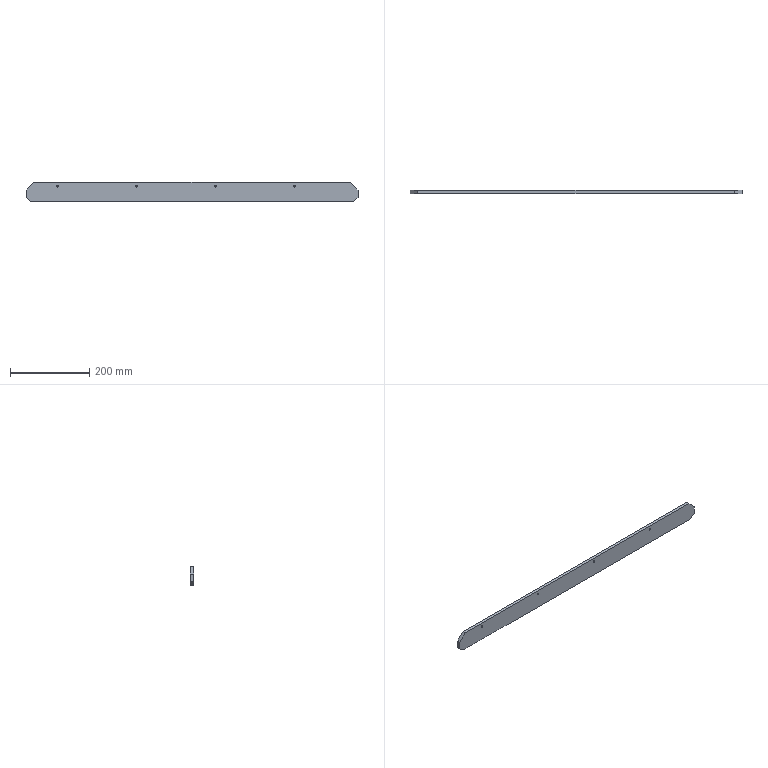Part | STEP file | PN_0038_chain guide rail_default_machined_ | 1 solid | 18 faces | box 840 x 8 x 50 mm | volume 330972 mm3 | plane 10 | cylinder 8 | commonest cylinder face diameters 5 x8
STEP:
#1=CARTESIAN_POINT('',(0.,0.,0.));
#2=DIRECTION('',(0.,0.,1.));
#3=DIRECTION('',(1.,0.,0.));
#4=AXIS2_PLACEMENT_3D('',#1,#2,#3);
#5=CARTESIAN_POINT('',(680.,-8.,-7.5));
#6=VERTEX_POINT('',#5);
#7=CARTESIAN_POINT('',(680.,0.,-7.5));
#8=VERTEX_POINT('',#7);
#9=CARTESIAN_POINT('',(680.,0.,-7.5));
#10=DIRECTION('',(0.,1.,0.));
#11=VECTOR('',#10,1.);
#12=LINE('',#9,#11);
#13=CARTESIAN_POINT('',(680.,0.,-10.));
#14=DIRECTION('',(0.,1.,0.));
#15=DIRECTION('',(0.,0.,1.));
#16=AXIS2_PLACEMENT_3D('',#13,#14,#15);
#17=CYLINDRICAL_SURFACE('',#16,2.5);
#18=CARTESIAN_POINT('',(6.283,0.));
#19=DIRECTION('',(0.,1.));
#20=VECTOR('',#19,1.);
#21=LINE('',#18,#20);
#22=(GEOMETRIC_REPRESENTATION_CONTEXT(2)PARAMETRIC_REPRESENTATION_CONTEXT()REPRESENTATION_CONTEXT('',''));
#23=DEFINITIONAL_REPRESENTATION('',(#21),#22);
#24=PCURVE('',#17,#23);
#25=CARTESIAN_POINT('',(680.,0.,-10.));
#26=DIRECTION('',(0.,1.,0.));
#27=DIRECTION('',(0.,0.,1.));
#28=AXIS2_PLACEMENT_3D('',#25,#26,#27);
#29=CYLINDRICAL_SURFACE('',#28,2.5);
#30=CARTESIAN_POINT('',(0.,0.));
#31=DIRECTION('',(0.,1.));
#32=VECTOR('',#31,1.);
#33=LINE('',#30,#32);
#34=(GEOMETRIC_REPRESENTATION_CONTEXT(2)PARAMETRIC_REPRESENTATION_CONTEXT()REPRESENTATION_CONTEXT('',''));
#35=DEFINITIONAL_REPRESENTATION('',(#33),#34);
#36=PCURVE('',#29,#35);
#37=SURFACE_CURVE('',#12,(#24,#36),.PCURVE_S1.);
#38=EDGE_CURVE('',#6,#8,#37,.T.);
#39=ORIENTED_EDGE('',*,*,#38,.T.);
#40=CARTESIAN_POINT('',(680.,0.,-12.5));
#41=VERTEX_POINT('',#40);
#42=CARTESIAN_POINT('',(680.,0.,-10.));
#43=DIRECTION('',(0.,-1.,0.));
#44=DIRECTION('',(0.,0.,1.));
#45=AXIS2_PLACEMENT_3D('',#42,#43,#44);
#46=CIRCLE('',#45,2.5);
#47=CARTESIAN_POINT('',(6.283,0.));
#48=DIRECTION('',(-1.,0.));
#49=VECTOR('',#48,1.);
#50=LINE('',#47,#49);
#51=(GEOMETRIC_REPRESENTATION_CONTEXT(2)PARAMETRIC_REPRESENTATION_CONTEXT()REPRESENTATION_CONTEXT('',''));
#52=DEFINITIONAL_REPRESENTATION('',(#50),#51);
#53=PCURVE('',#17,#52);
#54=CARTESIAN_POINT('',(0.,0.,0.));
#55=DIRECTION('',(0.,-1.,0.));
#56=DIRECTION('',(0.,0.,-1.));
#57=AXIS2_PLACEMENT_3D('',#54,#55,#56);
#58=PLANE('',#57);
#59=CARTESIAN_POINT('',(10.,680.));
#60=DIRECTION('',(-1.,0.));
#61=AXIS2_PLACEMENT_2D('',#59,#60);
#62=CIRCLE('',#61,2.5);
#63=(GEOMETRIC_REPRESENTATION_CONTEXT(2)PARAMETRIC_REPRESENTATION_CONTEXT()REPRESENTATION_CONTEXT('',''));
#64=DEFINITIONAL_REPRESENTATION('',(#62),#63);
#65=PCURVE('',#58,#64);
#66=SURFACE_CURVE('',#46,(#53,#65),.PCURVE_S1.);
#67=EDGE_CURVE('',#8,#41,#66,.T.);
#68=ORIENTED_EDGE('',*,*,#67,.T.);
#69=CARTESIAN_POINT('',(680.,-8.,-12.5));
#70=VERTEX_POINT('',#69);
#71=CARTESIAN_POINT('',(680.,0.,-12.5));
#72=DIRECTION('',(0.,1.,0.));
#73=VECTOR('',#72,1.);
#74=LINE('',#71,#73);
#75=CARTESIAN_POINT('',(3.142,0.));
#76=DIRECTION('',(0.,1.));
#77=VECTOR('',#76,1.);
#78=LINE('',#75,#77);
#79=(GEOMETRIC_REPRESENTATION_CONTEXT(2)PARAMETRIC_REPRESENTATION_CONTEXT()REPRESENTATION_CONTEXT('',''));
#80=DEFINITIONAL_REPRESENTATION('',(#78),#79);
#81=PCURVE('',#17,#80);
#82=CARTESIAN_POINT('',(3.142,0.));
#83=DIRECTION('',(0.,1.));
#84=VECTOR('',#83,1.);
#85=LINE('',#82,#84);
#86=(GEOMETRIC_REPRESENTATION_CONTEXT(2)PARAMETRIC_REPRESENTATION_CONTEXT()REPRESENTATION_CONTEXT('',''));
#87=DEFINITIONAL_REPRESENTATION('',(#85),#86);
#88=PCURVE('',#29,#87);
#89=SURFACE_CURVE('',#74,(#81,#88),.PCURVE_S1.);
#90=EDGE_CURVE('',#70,#41,#89,.T.);
#91=ORIENTED_EDGE('',*,*,#90,.F.);
#92=CARTESIAN_POINT('',(680.,-8.,-10.));
#93=DIRECTION('',(0.,1.,0.));
#94=DIRECTION('',(0.,0.,1.));
#95=AXIS2_PLACEMENT_3D('',#92,#93,#94);
#96=CIRCLE('',#95,2.5);
#97=CARTESIAN_POINT('',(0.,-8.));
#98=DIRECTION('',(1.,0.));
#99=VECTOR('',#98,1.);
#100=LINE('',#97,#99);
#101=(GEOMETRIC_REPRESENTATION_CONTEXT(2)PARAMETRIC_REPRESENTATION_CONTEXT()REPRESENTATION_CONTEXT('',''));
#102=DEFINITIONAL_REPRESENTATION('',(#100),#101);
#103=PCURVE('',#17,#102);
#104=CARTESIAN_POINT('',(0.,-8.,0.));
#105=DIRECTION('',(0.,-1.,0.));
#106=DIRECTION('',(0.,0.,-1.));
#107=AXIS2_PLACEMENT_3D('',#104,#105,#106);
#108=PLANE('',#107);
#109=CARTESIAN_POINT('',(7.5,680.));
#110=CARTESIAN_POINT('',(7.5,684.33));
#111=CARTESIAN_POINT('',(11.25,682.165));
#112=CARTESIAN_POINT('',(15.,680.));
#113=CARTESIAN_POINT('',(11.25,677.835));
#114=CARTESIAN_POINT('',(7.5,675.67));
#115=CARTESIAN_POINT('',(7.5,680.));
#116=(BOUNDED_CURVE()B_SPLINE_CURVE(2,(#109,#110,#111,#112,#113,#114,#115),.UNSPECIFIED.,.T.,.F.)B_SPLINE_CURVE_WITH_KNOTS((1,2,2,2,2,1),(-2.094,0.,2.094,4.189,6.283,8.378),.UNSPECIFIED.)CURVE()GEOMETRIC_REPRESENTATION_ITEM()RATIONAL_B_SPLINE_CURVE((1.,0.5,1.,0.5,1.,0.5,1.))REPRESENTATION_ITEM(''));
#117=(GEOMETRIC_REPRESENTATION_CONTEXT(2)PARAMETRIC_REPRESENTATION_CONTEXT()REPRESENTATION_CONTEXT('',''));
#118=DEFINITIONAL_REPRESENTATION('',(#116),#117);
#119=PCURVE('',#108,#118);
#120=SURFACE_CURVE('',#96,(#103,#119),.PCURVE_S1.);
#121=EDGE_CURVE('',#70,#6,#120,.T.);
#122=ORIENTED_EDGE('',*,*,#121,.T.);
#123=EDGE_LOOP('',(#39,#68,#91,#122));
#124=FACE_BOUND('',#123,.F.);
#125=ADVANCED_FACE('',(#124),#17,.F.);
#126=CARTESIAN_POINT('',(480.,-8.,-7.5));
#127=VERTEX_POINT('',#126);
#128=CARTESIAN_POINT('',(480.,0.,-7.5));
#129=VERTEX_POINT('',#128);
#130=CARTESIAN_POINT('',(480.,0.,-7.5));
#131=DIRECTION('',(0.,1.,0.));
#132=VECTOR('',#131,1.);
#133=LINE('',#130,#132);
#134=CARTESIAN_POINT('',(480.,0.,-10.));
#135=DIRECTION('',(0.,1.,0.));
#136=DIRECTION('',(0.,0.,1.));
#137=AXIS2_PLACEMENT_3D('',#134,#135,#136);
#138=CYLINDRICAL_SURFACE('',#137,2.5);
#139=CARTESIAN_POINT('',(6.283,0.));
#140=DIRECTION('',(0.,1.));
#141=VECTOR('',#140,1.);
#142=LINE('',#139,#141);
#143=(GEOMETRIC_REPRESENTATION_CONTEXT(2)PARAMETRIC_REPRESENTATION_CONTEXT()REPRESENTATION_CONTEXT('',''));
#144=DEFINITIONAL_REPRESENTATION('',(#142),#143);
#145=PCURVE('',#138,#144);
#146=CARTESIAN_POINT('',(480.,0.,-10.));
#147=DIRECTION('',(0.,1.,0.));
#148=DIRECTION('',(0.,0.,1.));
#149=AXIS2_PLACEMENT_3D('',#146,#147,#148);
#150=CYLINDRICAL_SURFACE('',#149,2.5);
#151=CARTESIAN_POINT('',(0.,0.));
#152=DIRECTION('',(0.,1.));
#153=VECTOR('',#152,1.);
#154=LINE('',#151,#153);
#155=(GEOMETRIC_REPRESENTATION_CONTEXT(2)PARAMETRIC_REPRESENTATION_CONTEXT()REPRESENTATION_CONTEXT('',''));
#156=DEFINITIONAL_REPRESENTATION('',(#154),#155);
#157=PCURVE('',#150,#156);
#158=SURFACE_CURVE('',#133,(#145,#157),.PCURVE_S1.);
#159=EDGE_CURVE('',#127,#129,#158,.T.);
#160=ORIENTED_EDGE('',*,*,#159,.T.);
#161=CARTESIAN_POINT('',(480.,0.,-12.5));
#162=VERTEX_POINT('',#161);
#163=CARTESIAN_POINT('',(480.,0.,-10.));
#164=DIRECTION('',(0.,-1.,0.));
#165=DIRECTION('',(0.,0.,1.));
#166=AXIS2_PLACEMENT_3D('',#163,#164,#165);
#167=CIRCLE('',#166,2.5);
#168=CARTESIAN_POINT('',(6.283,0.));
#169=DIRECTION('',(-1.,0.));
#170=VECTOR('',#169,1.);
#171=LINE('',#168,#170);
#172=(GEOMETRIC_REPRESENTATION_CONTEXT(2)PARAMETRIC_REPRESENTATION_CONTEXT()REPRESENTATION_CONTEXT('',''));
#173=DEFINITIONAL_REPRESENTATION('',(#171),#172);
#174=PCURVE('',#138,#173);
#175=CARTESIAN_POINT('',(10.,480.));
#176=DIRECTION('',(-1.,0.));
#177=AXIS2_PLACEMENT_2D('',#175,#176);
#178=CIRCLE('',#177,2.5);
#179=(GEOMETRIC_REPRESENTATION_CONTEXT(2)PARAMETRIC_REPRESENTATION_CONTEXT()REPRESENTATION_CONTEXT('',''));
#180=DEFINITIONAL_REPRESENTATION('',(#178),#179);
#181=PCURVE('',#58,#180);
#182=SURFACE_CURVE('',#167,(#174,#181),.PCURVE_S1.);
#183=EDGE_CURVE('',#129,#162,#182,.T.);
#184=ORIENTED_EDGE('',*,*,#183,.T.);
#185=CARTESIAN_POINT('',(480.,-8.,-12.5));
#186=VERTEX_POINT('',#185);
#187=CARTESIAN_POINT('',(480.,0.,-12.5));
#188=DIRECTION('',(0.,1.,0.));
#189=VECTOR('',#188,1.);
#190=LINE('',#187,#189);
#191=CARTESIAN_POINT('',(3.142,0.));
#192=DIRECTION('',(0.,1.));
#193=VECTOR('',#192,1.);
#194=LINE('',#191,#193);
#195=(GEOMETRIC_REPRESENTATION_CONTEXT(2)PARAMETRIC_REPRESENTATION_CONTEXT()REPRESENTATION_CONTEXT('',''));
#196=DEFINITIONAL_REPRESENTATION('',(#194),#195);
#197=PCURVE('',#138,#196);
#198=CARTESIAN_POINT('',(3.142,0.));
#199=DIRECTION('',(0.,1.));
#200=VECTOR('',#199,1.);
#201=LINE('',#198,#200);
#202=(GEOMETRIC_REPRESENTATION_CONTEXT(2)PARAMETRIC_REPRESENTATION_CONTEXT()REPRESENTATION_CONTEXT('',''));
#203=DEFINITIONAL_REPRESENTATION('',(#201),#202);
#204=PCURVE('',#150,#203);
#205=SURFACE_CURVE('',#190,(#197,#204),.PCURVE_S1.);
#206=EDGE_CURVE('',#186,#162,#205,.T.);
#207=ORIENTED_EDGE('',*,*,#206,.F.);
#208=CARTESIAN_POINT('',(480.,-8.,-10.));
#209=DIRECTION('',(0.,1.,0.));
#210=DIRECTION('',(0.,0.,1.));
#211=AXIS2_PLACEMENT_3D('',#208,#209,#210);
#212=CIRCLE('',#211,2.5);
#213=CARTESIAN_POINT('',(0.,-8.));
#214=DIRECTION('',(1.,0.));
#215=VECTOR('',#214,1.);
#216=LINE('',#213,#215);
#217=(GEOMETRIC_REPRESENTATION_CONTEXT(2)PARAMETRIC_REPRESENTATION_CONTEXT()REPRESENTATION_CONTEXT('',''));
#218=DEFINITIONAL_REPRESENTATION('',(#216),#217);
#219=PCURVE('',#138,#218);
#220=CARTESIAN_POINT('',(7.5,480.));
#221=CARTESIAN_POINT('',(7.5,484.33));
#222=CARTESIAN_POINT('',(11.25,482.165));
#223=CARTESIAN_POINT('',(15.,480.));
#224=CARTESIAN_POINT('',(11.25,477.835));
#225=CARTESIAN_POINT('',(7.5,475.67));
#226=CARTESIAN_POINT('',(7.5,480.));
#227=(BOUNDED_CURVE()B_SPLINE_CURVE(2,(#220,#221,#222,#223,#224,#225,#226),.UNSPECIFIED.,.T.,.F.)B_SPLINE_CURVE_WITH_KNOTS((1,2,2,2,2,1),(-2.094,0.,2.094,4.189,6.283,8.378),.UNSPECIFIED.)CURVE()GEOMETRIC_REPRESENTATION_ITEM()RATIONAL_B_SPLINE_CURVE((1.,0.5,1.,0.5,1.,0.5,1.))REPRESENTATION_ITEM(''));
#228=(GEOMETRIC_REPRESENTATION_CONTEXT(2)PARAMETRIC_REPRESENTATION_CONTEXT()REPRESENTATION_CONTEXT('',''));
#229=DEFINITIONAL_REPRESENTATION('',(#227),#228);
#230=PCURVE('',#108,#229);
#231=SURFACE_CURVE('',#212,(#219,#230),.PCURVE_S1.);
#232=EDGE_CURVE('',#186,#127,#231,.T.);
#233=ORIENTED_EDGE('',*,*,#232,.T.);
#234=EDGE_LOOP('',(#160,#184,#207,#233));
#235=FACE_BOUND('',#234,.F.);
#236=ADVANCED_FACE('',(#235),#138,.F.);
#237=CARTESIAN_POINT('',(80.,-8.,-7.5));
#238=VERTEX_POINT('',#237);
#239=CARTESIAN_POINT('',(80.,0.,-7.5));
#240=VERTEX_POINT('',#239);
#241=CARTESIAN_POINT('',(80.,0.,-7.5));
#242=DIRECTION('',(0.,1.,0.));
#243=VECTOR('',#242,1.);
#244=LINE('',#241,#243);
#245=CARTESIAN_POINT('',(80.,0.,-10.));
#246=DIRECTION('',(0.,1.,0.));
#247=DIRECTION('',(0.,0.,1.));
#248=AXIS2_PLACEMENT_3D('',#245,#246,#247);
#249=CYLINDRICAL_SURFACE('',#248,2.5);
#250=CARTESIAN_POINT('',(6.283,0.));
#251=DIRECTION('',(0.,1.));
#252=VECTOR('',#251,1.);
#253=LINE('',#250,#252);
#254=(GEOMETRIC_REPRESENTATION_CONTEXT(2)PARAMETRIC_REPRESENTATION_CONTEXT()REPRESENTATION_CONTEXT('',''));
#255=DEFINITIONAL_REPRESENTATION('',(#253),#254);
#256=PCURVE('',#249,#255);
#257=CARTESIAN_POINT('',(80.,0.,-10.));
#258=DIRECTION('',(0.,1.,0.));
#259=DIRECTION('',(0.,0.,1.));
#260=AXIS2_PLACEMENT_3D('',#257,#258,#259);
#261=CYLINDRICAL_SURFACE('',#260,2.5);
#262=CARTESIAN_POINT('',(0.,0.));
#263=DIRECTION('',(0.,1.));
#264=VECTOR('',#263,1.);
#265=LINE('',#262,#264);
#266=(GEOMETRIC_REPRESENTATION_CONTEXT(2)PARAMETRIC_REPRESENTATION_CONTEXT()REPRESENTATION_CONTEXT('',''));
#267=DEFINITIONAL_REPRESENTATION('',(#265),#266);
#268=PCURVE('',#261,#267);
#269=SURFACE_CURVE('',#244,(#256,#268),.PCURVE_S1.);
#270=EDGE_CURVE('',#238,#240,#269,.T.);
#271=ORIENTED_EDGE('',*,*,#270,.T.);
#272=CARTESIAN_POINT('',(80.,0.,-12.5));
#273=VERTEX_POINT('',#272);
#274=CARTESIAN_POINT('',(80.,0.,-10.));
#275=DIRECTION('',(0.,-1.,0.));
#276=DIRECTION('',(0.,0.,1.));
#277=AXIS2_PLACEMENT_3D('',#274,#275,#276);
#278=CIRCLE('',#277,2.5);
#279=CARTESIAN_POINT('',(6.283,0.));
#280=DIRECTION('',(-1.,0.));
#281=VECTOR('',#280,1.);
#282=LINE('',#279,#281);
#283=(GEOMETRIC_REPRESENTATION_CONTEXT(2)PARAMETRIC_REPRESENTATION_CONTEXT()REPRESENTATION_CONTEXT('',''));
#284=DEFINITIONAL_REPRESENTATION('',(#282),#283);
#285=PCURVE('',#249,#284);
#286=CARTESIAN_POINT('',(10.,80.));
#287=DIRECTION('',(-1.,0.));
#288=AXIS2_PLACEMENT_2D('',#286,#287);
#289=CIRCLE('',#288,2.5);
#290=(GEOMETRIC_REPRESENTATION_CONTEXT(2)PARAMETRIC_REPRESENTATION_CONTEXT()REPRESENTATION_CONTEXT('',''));
#291=DEFINITIONAL_REPRESENTATION('',(#289),#290);
#292=PCURVE('',#58,#291);
#293=SURFACE_CURVE('',#278,(#285,#292),.PCURVE_S1.);
#294=EDGE_CURVE('',#240,#273,#293,.T.);
#295=ORIENTED_EDGE('',*,*,#294,.T.);
#296=CARTESIAN_POINT('',(80.,-8.,-12.5));
#297=VERTEX_POINT('',#296);
#298=CARTESIAN_POINT('',(80.,0.,-12.5));
#299=DIRECTION('',(0.,1.,0.));
#300=VECTOR('',#299,1.);
#301=LINE('',#298,#300);
#302=CARTESIAN_POINT('',(3.142,0.));
#303=DIRECTION('',(0.,1.));
#304=VECTOR('',#303,1.);
#305=LINE('',#302,#304);
#306=(GEOMETRIC_REPRESENTATION_CONTEXT(2)PARAMETRIC_REPRESENTATION_CONTEXT()REPRESENTATION_CONTEXT('',''));
#307=DEFINITIONAL_REPRESENTATION('',(#305),#306);
#308=PCURVE('',#249,#307);
#309=CARTESIAN_POINT('',(3.142,0.));
#310=DIRECTION('',(0.,1.));
#311=VECTOR('',#310,1.);
#312=LINE('',#309,#311);
#313=(GEOMETRIC_REPRESENTATION_CONTEXT(2)PARAMETRIC_REPRESENTATION_CONTEXT()REPRESENTATION_CONTEXT('',''));
#314=DEFINITIONAL_REPRESENTATION('',(#312),#313);
#315=PCURVE('',#261,#314);
#316=SURFACE_CURVE('',#301,(#308,#315),.PCURVE_S1.);
#317=EDGE_CURVE('',#297,#273,#316,.T.);
#318=ORIENTED_EDGE('',*,*,#317,.F.);
#319=CARTESIAN_POINT('',(80.,-8.,-10.));
#320=DIRECTION('',(0.,1.,0.));
#321=DIRECTION('',(0.,0.,1.));
#322=AXIS2_PLACEMENT_3D('',#319,#320,#321);
#323=CIRCLE('',#322,2.5);
#324=CARTESIAN_POINT('',(0.,-8.));
#325=DIRECTION('',(1.,0.));
#326=VECTOR('',#325,1.);
#327=LINE('',#324,#326);
#328=(GEOMETRIC_REPRESENTATION_CONTEXT(2)PARAMETRIC_REPRESENTATION_CONTEXT()REPRESENTATION_CONTEXT('',''));
#329=DEFINITIONAL_REPRESENTATION('',(#327),#328);
#330=PCURVE('',#249,#329);
#331=CARTESIAN_POINT('',(7.5,80.));
#332=CARTESIAN_POINT('',(7.5,84.33));
#333=CARTESIAN_POINT('',(11.25,82.165));
#334=CARTESIAN_POINT('',(15.,80.));
#335=CARTESIAN_POINT('',(11.25,77.835));
#336=CARTESIAN_POINT('',(7.5,75.67));
#337=CARTESIAN_POINT('',(7.5,80.));
#338=(BOUNDED_CURVE()B_SPLINE_CURVE(2,(#331,#332,#333,#334,#335,#336,#337),.UNSPECIFIED.,.T.,.F.)B_SPLINE_CURVE_WITH_KNOTS((1,2,2,2,2,1),(-2.094,0.,2.094,4.189,6.283,8.378),.UNSPECIFIED.)CURVE()GEOMETRIC_REPRESENTATION_ITEM()RATIONAL_B_SPLINE_CURVE((1.,0.5,1.,0.5,1.,0.5,1.))REPRESENTATION_ITEM(''));
#339=(GEOMETRIC_REPRESENTATION_CONTEXT(2)PARAMETRIC_REPRESENTATION_CONTEXT()REPRESENTATION_CONTEXT('',''));
#340=DEFINITIONAL_REPRESENTATION('',(#338),#339);
#341=PCURVE('',#108,#340);
#342=SURFACE_CURVE('',#323,(#330,#341),.PCURVE_S1.);
#343=EDGE_CURVE('',#297,#238,#342,.T.);
#344=ORIENTED_EDGE('',*,*,#343,.T.);
#345=EDGE_LOOP('',(#271,#295,#318,#344));
#346=FACE_BOUND('',#345,.F.);
#347=ADVANCED_FACE('',(#346),#249,.F.);
#348=CARTESIAN_POINT('',(280.,-8.,-7.5));
#349=VERTEX_POINT('',#348);
#350=CARTESIAN_POINT('',(280.,0.,-7.5));
#351=VERTEX_POINT('',#350);
#352=CARTESIAN_POINT('',(280.,0.,-7.5));
#353=DIRECTION('',(0.,1.,0.));
#354=VECTOR('',#353,1.);
#355=LINE('',#352,#354);
#356=CARTESIAN_POINT('',(280.,0.,-10.));
#357=DIRECTION('',(0.,1.,0.));
#358=DIRECTION('',(0.,0.,1.));
#359=AXIS2_PLACEMENT_3D('',#356,#357,#358);
#360=CYLINDRICAL_SURFACE('',#359,2.5);
#361=CARTESIAN_POINT('',(6.283,0.));
#362=DIRECTION('',(0.,1.));
#363=VECTOR('',#362,1.);
#364=LINE('',#361,#363);
#365=(GEOMETRIC_REPRESENTATION_CONTEXT(2)PARAMETRIC_REPRESENTATION_CONTEXT()REPRESENTATION_CONTEXT('',''));
#366=DEFINITIONAL_REPRESENTATION('',(#364),#365);
#367=PCURVE('',#360,#366);
#368=CARTESIAN_POINT('',(280.,0.,-10.));
#369=DIRECTION('',(0.,1.,0.));
#370=DIRECTION('',(0.,0.,1.));
#371=AXIS2_PLACEMENT_3D('',#368,#369,#370);
#372=CYLINDRICAL_SURFACE('',#371,2.5);
#373=CARTESIAN_POINT('',(0.,0.));
#374=DIRECTION('',(0.,1.));
#375=VECTOR('',#374,1.);
#376=LINE('',#373,#375);
#377=(GEOMETRIC_REPRESENTATION_CONTEXT(2)PARAMETRIC_REPRESENTATION_CONTEXT()REPRESENTATION_CONTEXT('',''));
#378=DEFINITIONAL_REPRESENTATION('',(#376),#377);
#379=PCURVE('',#372,#378);
#380=SURFACE_CURVE('',#355,(#367,#379),.PCURVE_S1.);
#381=EDGE_CURVE('',#349,#351,#380,.T.);
#382=ORIENTED_EDGE('',*,*,#381,.T.);
#383=CARTESIAN_POINT('',(280.,0.,-12.5));
#384=VERTEX_POINT('',#383);
#385=CARTESIAN_POINT('',(280.,0.,-10.));
#386=DIRECTION('',(0.,-1.,0.));
#387=DIRECTION('',(0.,0.,1.));
#388=AXIS2_PLACEMENT_3D('',#385,#386,#387);
#389=CIRCLE('',#388,2.5);
#390=CARTESIAN_POINT('',(6.283,0.));
#391=DIRECTION('',(-1.,0.));
#392=VECTOR('',#391,1.);
#393=LINE('',#390,#392);
#394=(GEOMETRIC_REPRESENTATION_CONTEXT(2)PARAMETRIC_REPRESENTATION_CONTEXT()REPRESENTATION_CONTEXT('',''));
#395=DEFINITIONAL_REPRESENTATION('',(#393),#394);
#396=PCURVE('',#360,#395);
#397=CARTESIAN_POINT('',(10.,280.));
#398=DIRECTION('',(-1.,0.));
#399=AXIS2_PLACEMENT_2D('',#397,#398);
#400=CIRCLE('',#399,2.5);
#401=(GEOMETRIC_REPRESENTATION_CONTEXT(2)PARAMETRIC_REPRESENTATION_CONTEXT()REPRESENTATION_CONTEXT('',''));
#402=DEFINITIONAL_REPRESENTATION('',(#400),#401);
#403=PCURVE('',#58,#402);
#404=SURFACE_CURVE('',#389,(#396,#403),.PCURVE_S1.);
#405=EDGE_CURVE('',#351,#384,#404,.T.);
#406=ORIENTED_EDGE('',*,*,#405,.T.);
#407=CARTESIAN_POINT('',(280.,-8.,-12.5));
#408=VERTEX_POINT('',#407);
#409=CARTESIAN_POINT('',(280.,0.,-12.5));
#410=DIRECTION('',(0.,1.,0.));
#411=VECTOR('',#410,1.);
#412=LINE('',#409,#411);
#413=CARTESIAN_POINT('',(3.142,0.));
#414=DIRECTION('',(0.,1.));
#415=VECTOR('',#414,1.);
#416=LINE('',#413,#415);
#417=(GEOMETRIC_REPRESENTATION_CONTEXT(2)PARAMETRIC_REPRESENTATION_CONTEXT()REPRESENTATION_CONTEXT('',''));
#418=DEFINITIONAL_REPRESENTATION('',(#416),#417);
#419=PCURVE('',#360,#418);
#420=CARTESIAN_POINT('',(3.142,0.));
#421=DIRECTION('',(0.,1.));
#422=VECTOR('',#421,1.);
#423=LINE('',#420,#422);
#424=(GEOMETRIC_REPRESENTATION_CONTEXT(2)PARAMETRIC_REPRESENTATION_CONTEXT()REPRESENTATION_CONTEXT('',''));
#425=DEFINITIONAL_REPRESENTATION('',(#423),#424);
#426=PCURVE('',#372,#425);
#427=SURFACE_CURVE('',#412,(#419,#426),.PCURVE_S1.);
#428=EDGE_CURVE('',#408,#384,#427,.T.);
#429=ORIENTED_EDGE('',*,*,#428,.F.);
#430=CARTESIAN_POINT('',(280.,-8.,-10.));
#431=DIRECTION('',(0.,1.,0.));
#432=DIRECTION('',(0.,0.,1.));
#433=AXIS2_PLACEMENT_3D('',#430,#431,#432);
#434=CIRCLE('',#433,2.5);
#435=CARTESIAN_POINT('',(0.,-8.));
#436=DIRECTION('',(1.,0.));
#437=VECTOR('',#436,1.);
#438=LINE('',#435,#437);
#439=(GEOMETRIC_REPRESENTATION_CONTEXT(2)PARAMETRIC_REPRESENTATION_CONTEXT()REPRESENTATION_CONTEXT('',''));
#440=DEFINITIONAL_REPRESENTATION('',(#438),#439);
#441=PCURVE('',#360,#440);
#442=CARTESIAN_POINT('',(7.5,280.));
#443=CARTESIAN_POINT('',(7.5,284.33));
#444=CARTESIAN_POINT('',(11.25,282.165));
#445=CARTESIAN_POINT('',(15.,280.));
#446=CARTESIAN_POINT('',(11.25,277.835));
#447=CARTESIAN_POINT('',(7.5,275.67));
#448=CARTESIAN_POINT('',(7.5,280.));
#449=(BOUNDED_CURVE()B_SPLINE_CURVE(2,(#442,#443,#444,#445,#446,#447,#448),.UNSPECIFIED.,.T.,.F.)B_SPLINE_CURVE_WITH_KNOTS((1,2,2,2,2,1),(-2.094,0.,2.094,4.189,6.283,8.378),.UNSPECIFIED.)CURVE()GEOMETRIC_REPRESENTATION_ITEM()RATIONAL_B_SPLINE_CURVE((1.,0.5,1.,0.5,1.,0.5,1.))REPRESENTATION_ITEM(''));
#450=(GEOMETRIC_REPRESENTATION_CONTEXT(2)PARAMETRIC_REPRESENTATION_CONTEXT()REPRESENTATION_CONTEXT('',''));
#451=DEFINITIONAL_REPRESENTATION('',(#449),#450);
#452=PCURVE('',#108,#451);
#453=SURFACE_CURVE('',#434,(#441,#452),.PCURVE_S1.);
#454=EDGE_CURVE('',#408,#349,#453,.T.);
#455=ORIENTED_EDGE('',*,*,#454,.T.);
#456=EDGE_LOOP('',(#382,#406,#429,#455));
#457=FACE_BOUND('',#456,.F.);
#458=ADVANCED_FACE('',(#457),#360,.F.);
#459=CARTESIAN_POINT('',(680.,-8.,-10.));
#460=DIRECTION('',(0.,1.,0.));
#461=DIRECTION('',(0.,0.,1.));
#462=AXIS2_PLACEMENT_3D('',#459,#460,#461);
#463=CIRCLE('',#462,2.5);
#464=CARTESIAN_POINT('',(7.5,680.));
#465=CARTESIAN_POINT('',(7.5,684.33));
#466=CARTESIAN_POINT('',(11.25,682.165));
#467=CARTESIAN_POINT('',(15.,680.));
#468=CARTESIAN_POINT('',(11.25,677.835));
#469=CARTESIAN_POINT('',(7.5,675.67));
#470=CARTESIAN_POINT('',(7.5,680.));
#471=(BOUNDED_CURVE()B_SPLINE_CURVE(2,(#464,#465,#466,#467,#468,#469,#470),.UNSPECIFIED.,.T.,.F.)B_SPLINE_CURVE_WITH_KNOTS((1,2,2,2,2,1),(-2.094,0.,2.094,4.189,6.283,8.378),.UNSPECIFIED.)CURVE()GEOMETRIC_REPRESENTATION_ITEM()RATIONAL_B_SPLINE_CURVE((1.,0.5,1.,0.5,1.,0.5,1.))REPRESENTATION_ITEM(''));
#472=(GEOMETRIC_REPRESENTATION_CONTEXT(2)PARAMETRIC_REPRESENTATION_CONTEXT()REPRESENTATION_CONTEXT('',''));
#473=DEFINITIONAL_REPRESENTATION('',(#471),#472);
#474=PCURVE('',#108,#473);
#475=CARTESIAN_POINT('',(0.,-8.));
#476=DIRECTION('',(1.,0.));
#477=VECTOR('',#476,1.);
#478=LINE('',#475,#477);
#479=(GEOMETRIC_REPRESENTATION_CONTEXT(2)PARAMETRIC_REPRESENTATION_CONTEXT()REPRESENTATION_CONTEXT('',''));
#480=DEFINITIONAL_REPRESENTATION('',(#478),#479);
#481=PCURVE('',#29,#480);
#482=SURFACE_CURVE('',#463,(#474,#481),.PCURVE_S1.);
#483=EDGE_CURVE('',#6,#70,#482,.T.);
#484=ORIENTED_EDGE('',*,*,#483,.T.);
#485=ORIENTED_EDGE('',*,*,#121,.T.);
#486=EDGE_LOOP('',(#484,#485));
#487=FACE_BOUND('',#486,.T.);
#488=CARTESIAN_POINT('',(480.,-8.,-10.));
#489=DIRECTION('',(0.,1.,0.));
#490=DIRECTION('',(0.,0.,1.));
#491=AXIS2_PLACEMENT_3D('',#488,#489,#490);
#492=CIRCLE('',#491,2.5);
#493=CARTESIAN_POINT('',(7.5,480.));
#494=CARTESIAN_POINT('',(7.5,484.33));
#495=CARTESIAN_POINT('',(11.25,482.165));
#496=CARTESIAN_POINT('',(15.,480.));
#497=CARTESIAN_POINT('',(11.25,477.835));
#498=CARTESIAN_POINT('',(7.5,475.67));
#499=CARTESIAN_POINT('',(7.5,480.));
#500=(BOUNDED_CURVE()B_SPLINE_CURVE(2,(#493,#494,#495,#496,#497,#498,#499),.UNSPECIFIED.,.T.,.F.)B_SPLINE_CURVE_WITH_KNOTS((1,2,2,2,2,1),(-2.094,0.,2.094,4.189,6.283,8.378),.UNSPECIFIED.)CURVE()GEOMETRIC_REPRESENTATION_ITEM()RATIONAL_B_SPLINE_CURVE((1.,0.5,1.,0.5,1.,0.5,1.))REPRESENTATION_ITEM(''));
#501=(GEOMETRIC_REPRESENTATION_CONTEXT(2)PARAMETRIC_REPRESENTATION_CONTEXT()REPRESENTATION_CONTEXT('',''));
#502=DEFINITIONAL_REPRESENTATION('',(#500),#501);
#503=PCURVE('',#108,#502);
#504=CARTESIAN_POINT('',(0.,-8.));
#505=DIRECTION('',(1.,0.));
#506=VECTOR('',#505,1.);
#507=LINE('',#504,#506);
#508=(GEOMETRIC_REPRESENTATION_CONTEXT(2)PARAMETRIC_REPRESENTATION_CONTEXT()REPRESENTATION_CONTEXT('',''));
#509=DEFINITIONAL_REPRESENTATION('',(#507),#508);
#510=PCURVE('',#150,#509);
#511=SURFACE_CURVE('',#492,(#503,#510),.PCURVE_S1.);
#512=EDGE_CURVE('',#127,#186,#511,.T.);
#513=ORIENTED_EDGE('',*,*,#512,.T.);
#514=ORIENTED_EDGE('',*,*,#232,.T.);
#515=EDGE_LOOP('',(#513,#514));
#516=FACE_BOUND('',#515,.T.);
#517=CARTESIAN_POINT('',(820.,-8.,0.));
#518=VERTEX_POINT('',#517);
#519=CARTESIAN_POINT('',(20.,-8.,0.));
#520=VERTEX_POINT('',#519);
#521=CARTESIAN_POINT('',(0.,-8.,0.));
#522=DIRECTION('',(-1.,0.,0.));
#523=VECTOR('',#522,1.);
#524=LINE('',#521,#523);
#525=CARTESIAN_POINT('',(0.,0.));
#526=DIRECTION('',(0.,-1.));
#527=VECTOR('',#526,1.);
#528=LINE('',#525,#527);
#529=(GEOMETRIC_REPRESENTATION_CONTEXT(2)PARAMETRIC_REPRESENTATION_CONTEXT()REPRESENTATION_CONTEXT('',''));
#530=DEFINITIONAL_REPRESENTATION('',(#528),#529);
#531=PCURVE('',#108,#530);
#532=CARTESIAN_POINT('',(0.,-8.,0.));
#533=DIRECTION('',(0.,0.,1.));
#534=DIRECTION('',(1.,0.,0.));
#535=AXIS2_PLACEMENT_3D('',#532,#533,#534);
#536=PLANE('',#535);
#537=CARTESIAN_POINT('',(0.,0.));
#538=DIRECTION('',(-1.,0.));
#539=VECTOR('',#538,1.);
#540=LINE('',#537,#539);
#541=(GEOMETRIC_REPRESENTATION_CONTEXT(2)PARAMETRIC_REPRESENTATION_CONTEXT()REPRESENTATION_CONTEXT('',''));
#542=DEFINITIONAL_REPRESENTATION('',(#540),#541);
#543=PCURVE('',#536,#542);
#544=SURFACE_CURVE('',#524,(#531,#543),.PCURVE_S1.);
#545=EDGE_CURVE('',#518,#520,#544,.T.);
#546=ORIENTED_EDGE('',*,*,#545,.T.);
#547=CARTESIAN_POINT('',(0.,-8.,-20.));
#548=VERTEX_POINT('',#547);
#549=CARTESIAN_POINT('',(20.,-8.,0.));
#550=DIRECTION('',(-0.7071,0.,-0.7071));
#551=VECTOR('',#550,1.);
#552=LINE('',#549,#551);
#553=CARTESIAN_POINT('',(0.,20.));
#554=DIRECTION('',(0.7071,-0.7071));
#555=VECTOR('',#554,1.);
#556=LINE('',#553,#555);
#557=(GEOMETRIC_REPRESENTATION_CONTEXT(2)PARAMETRIC_REPRESENTATION_CONTEXT()REPRESENTATION_CONTEXT('',''));
#558=DEFINITIONAL_REPRESENTATION('',(#556),#557);
#559=PCURVE('',#108,#558);
#560=CARTESIAN_POINT('',(0.,-8.,-20.));
#561=DIRECTION('',(0.7071,0.,-0.7071));
#562=DIRECTION('',(-0.7071,0.,-0.7071));
#563=AXIS2_PLACEMENT_3D('',#560,#561,#562);
#564=PLANE('',#563);
#565=CARTESIAN_POINT('',(-28.284,0.));
#566=DIRECTION('',(1.,0.));
#567=VECTOR('',#566,1.);
#568=LINE('',#565,#567);
#569=(GEOMETRIC_REPRESENTATION_CONTEXT(2)PARAMETRIC_REPRESENTATION_CONTEXT()REPRESENTATION_CONTEXT('',''));
#570=DEFINITIONAL_REPRESENTATION('',(#568),#569);
#571=PCURVE('',#564,#570);
#572=SURFACE_CURVE('',#552,(#559,#571),.PCURVE_S1.);
#573=EDGE_CURVE('',#520,#548,#572,.T.);
#574=ORIENTED_EDGE('',*,*,#573,.T.);
#575=CARTESIAN_POINT('',(0.,-8.,-40.));
#576=VERTEX_POINT('',#575);
#577=CARTESIAN_POINT('',(0.,-8.,0.));
#578=DIRECTION('',(0.,0.,-1.));
#579=VECTOR('',#578,1.);
#580=LINE('',#577,#579);
#581=CARTESIAN_POINT('',(0.,0.));
#582=DIRECTION('',(1.,0.));
#583=VECTOR('',#582,1.);
#584=LINE('',#581,#583);
#585=(GEOMETRIC_REPRESENTATION_CONTEXT(2)PARAMETRIC_REPRESENTATION_CONTEXT()REPRESENTATION_CONTEXT('',''));
#586=DEFINITIONAL_REPRESENTATION('',(#584),#585);
#587=PCURVE('',#108,#586);
#588=CARTESIAN_POINT('',(0.,-8.,0.));
#589=DIRECTION('',(-1.,0.,0.));
#590=DIRECTION('',(0.,0.,1.));
#591=AXIS2_PLACEMENT_3D('',#588,#589,#590);
#592=PLANE('',#591);
#593=CARTESIAN_POINT('',(0.,0.));
#594=DIRECTION('',(-1.,0.));
#595=VECTOR('',#594,1.);
#596=LINE('',#593,#595);
#597=(GEOMETRIC_REPRESENTATION_CONTEXT(2)PARAMETRIC_REPRESENTATION_CONTEXT()REPRESENTATION_CONTEXT('',''));
#598=DEFINITIONAL_REPRESENTATION('',(#596),#597);
#599=PCURVE('',#592,#598);
#600=SURFACE_CURVE('',#580,(#587,#599),.PCURVE_S1.);
#601=EDGE_CURVE('',#548,#576,#600,.T.);
#602=ORIENTED_EDGE('',*,*,#601,.T.);
#603=CARTESIAN_POINT('',(15.,-8.,-50.));
#604=VERTEX_POINT('',#603);
#605=CARTESIAN_POINT('',(0.,-8.,-40.));
#606=DIRECTION('',(0.8321,0.,-0.5547));
#607=VECTOR('',#606,1.);
#608=LINE('',#605,#607);
#609=CARTESIAN_POINT('',(40.,0.));
#610=DIRECTION('',(0.5547,0.8321));
#611=VECTOR('',#610,1.);
#612=LINE('',#609,#611);
#613=(GEOMETRIC_REPRESENTATION_CONTEXT(2)PARAMETRIC_REPRESENTATION_CONTEXT()REPRESENTATION_CONTEXT('',''));
#614=DEFINITIONAL_REPRESENTATION('',(#612),#613);
#615=PCURVE('',#108,#614);
#616=CARTESIAN_POINT('',(15.,-8.,-50.));
#617=DIRECTION('',(0.5547,0.,0.8321));
#618=DIRECTION('',(0.8321,0.,-0.5547));
#619=AXIS2_PLACEMENT_3D('',#616,#617,#618);
#620=PLANE('',#619);
#621=CARTESIAN_POINT('',(-18.028,0.));
#622=DIRECTION('',(1.,0.));
#623=VECTOR('',#622,1.);
#624=LINE('',#621,#623);
#625=(GEOMETRIC_REPRESENTATION_CONTEXT(2)PARAMETRIC_REPRESENTATION_CONTEXT()REPRESENTATION_CONTEXT('',''));
#626=DEFINITIONAL_REPRESENTATION('',(#624),#625);
#627=PCURVE('',#620,#626);
#628=SURFACE_CURVE('',#608,(#615,#627),.PCURVE_S1.);
#629=EDGE_CURVE('',#576,#604,#628,.T.);
#630=ORIENTED_EDGE('',*,*,#629,.T.);
#631=CARTESIAN_POINT('',(825.,-8.,-50.));
#632=VERTEX_POINT('',#631);
#633=CARTESIAN_POINT('',(0.,-8.,-50.));
#634=DIRECTION('',(1.,0.,0.));
#635=VECTOR('',#634,1.);
#636=LINE('',#633,#635);
#637=CARTESIAN_POINT('',(50.,0.));
#638=DIRECTION('',(0.,1.));
#639=VECTOR('',#638,1.);
#640=LINE('',#637,#639);
#641=(GEOMETRIC_REPRESENTATION_CONTEXT(2)PARAMETRIC_REPRESENTATION_CONTEXT()REPRESENTATION_CONTEXT('',''));
#642=DEFINITIONAL_REPRESENTATION('',(#640),#641);
#643=PCURVE('',#108,#642);
#644=CARTESIAN_POINT('',(0.,-8.,-50.));
#645=DIRECTION('',(0.,0.,-1.));
#646=DIRECTION('',(-1.,0.,0.));
#647=AXIS2_PLACEMENT_3D('',#644,#645,#646);
#648=PLANE('',#647);
#649=CARTESIAN_POINT('',(0.,0.));
#650=DIRECTION('',(-1.,0.));
#651=VECTOR('',#650,1.);
#652=LINE('',#649,#651);
#653=(GEOMETRIC_REPRESENTATION_CONTEXT(2)PARAMETRIC_REPRESENTATION_CONTEXT()REPRESENTATION_CONTEXT('',''));
#654=DEFINITIONAL_REPRESENTATION('',(#652),#653);
#655=PCURVE('',#648,#654);
#656=SURFACE_CURVE('',#636,(#643,#655),.PCURVE_S1.);
#657=EDGE_CURVE('',#604,#632,#656,.T.);
#658=ORIENTED_EDGE('',*,*,#657,.T.);
#659=CARTESIAN_POINT('',(840.,-8.,-40.));
#660=VERTEX_POINT('',#659);
#661=CARTESIAN_POINT('',(825.,-8.,-50.));
#662=DIRECTION('',(0.8321,0.,0.5547));
#663=VECTOR('',#662,1.);
#664=LINE('',#661,#663);
#665=CARTESIAN_POINT('',(50.,825.));
#666=DIRECTION('',(-0.5547,0.8321));
#667=VECTOR('',#666,1.);
#668=LINE('',#665,#667);
#669=(GEOMETRIC_REPRESENTATION_CONTEXT(2)PARAMETRIC_REPRESENTATION_CONTEXT()REPRESENTATION_CONTEXT('',''));
#670=DEFINITIONAL_REPRESENTATION('',(#668),#669);
#671=PCURVE('',#108,#670);
#672=CARTESIAN_POINT('',(840.,-8.,-40.));
#673=DIRECTION('',(-0.5547,0.,0.8321));
#674=DIRECTION('',(0.8321,0.,0.5547));
#675=AXIS2_PLACEMENT_3D('',#672,#673,#674);
#676=PLANE('',#675);
#677=CARTESIAN_POINT('',(-18.028,0.));
#678=DIRECTION('',(1.,0.));
#679=VECTOR('',#678,1.);
#680=LINE('',#677,#679);
#681=(GEOMETRIC_REPRESENTATION_CONTEXT(2)PARAMETRIC_REPRESENTATION_CONTEXT()REPRESENTATION_CONTEXT('',''));
#682=DEFINITIONAL_REPRESENTATION('',(#680),#681);
#683=PCURVE('',#676,#682);
#684=SURFACE_CURVE('',#664,(#671,#683),.PCURVE_S1.);
#685=EDGE_CURVE('',#632,#660,#684,.T.);
#686=ORIENTED_EDGE('',*,*,#685,.T.);
#687=CARTESIAN_POINT('',(840.,-8.,-20.));
#688=VERTEX_POINT('',#687);
#689=CARTESIAN_POINT('',(840.,-8.,0.));
#690=DIRECTION('',(0.,0.,1.));
#691=VECTOR('',#690,1.);
#692=LINE('',#689,#691);
#693=CARTESIAN_POINT('',(0.,840.));
#694=DIRECTION('',(-1.,0.));
#695=VECTOR('',#694,1.);
#696=LINE('',#693,#695);
#697=(GEOMETRIC_REPRESENTATION_CONTEXT(2)PARAMETRIC_REPRESENTATION_CONTEXT()REPRESENTATION_CONTEXT('',''));
#698=DEFINITIONAL_REPRESENTATION('',(#696),#697);
#699=PCURVE('',#108,#698);
#700=CARTESIAN_POINT('',(840.,-8.,0.));
#701=DIRECTION('',(1.,0.,0.));
#702=DIRECTION('',(0.,0.,-1.));
#703=AXIS2_PLACEMENT_3D('',#700,#701,#702);
#704=PLANE('',#703);
#705=CARTESIAN_POINT('',(0.,0.));
#706=DIRECTION('',(-1.,0.));
#707=VECTOR('',#706,1.);
#708=LINE('',#705,#707);
#709=(GEOMETRIC_REPRESENTATION_CONTEXT(2)PARAMETRIC_REPRESENTATION_CONTEXT()REPRESENTATION_CONTEXT('',''));
#710=DEFINITIONAL_REPRESENTATION('',(#708),#709);
#711=PCURVE('',#704,#710);
#712=SURFACE_CURVE('',#692,(#699,#711),.PCURVE_S1.);
#713=EDGE_CURVE('',#660,#688,#712,.T.);
#714=ORIENTED_EDGE('',*,*,#713,.T.);
#715=CARTESIAN_POINT('',(840.,-8.,-20.));
#716=DIRECTION('',(-0.7071,0.,0.7071));
#717=VECTOR('',#716,1.);
#718=LINE('',#715,#717);
#719=CARTESIAN_POINT('',(20.,840.));
#720=DIRECTION('',(-0.7071,-0.7071));
#721=VECTOR('',#720,1.);
#722=LINE('',#719,#721);
#723=(GEOMETRIC_REPRESENTATION_CONTEXT(2)PARAMETRIC_REPRESENTATION_CONTEXT()REPRESENTATION_CONTEXT('',''));
#724=DEFINITIONAL_REPRESENTATION('',(#722),#723);
#725=PCURVE('',#108,#724);
#726=CARTESIAN_POINT('',(820.,-8.,0.));
#727=DIRECTION('',(-0.7071,0.,-0.7071));
#728=DIRECTION('',(-0.7071,0.,0.7071));
#729=AXIS2_PLACEMENT_3D('',#726,#727,#728);
#730=PLANE('',#729);
#731=CARTESIAN_POINT('',(-28.284,0.));
#732=DIRECTION('',(1.,0.));
#733=VECTOR('',#732,1.);
#734=LINE('',#731,#733);
#735=(GEOMETRIC_REPRESENTATION_CONTEXT(2)PARAMETRIC_REPRESENTATION_CONTEXT()REPRESENTATION_CONTEXT('',''));
#736=DEFINITIONAL_REPRESENTATION('',(#734),#735);
#737=PCURVE('',#730,#736);
#738=SURFACE_CURVE('',#718,(#725,#737),.PCURVE_S1.);
#739=EDGE_CURVE('',#688,#518,#738,.T.);
#740=ORIENTED_EDGE('',*,*,#739,.T.);
#741=EDGE_LOOP('',(#546,#574,#602,#630,#658,#686,#714,#740));
#742=FACE_BOUND('',#741,.T.);
#743=CARTESIAN_POINT('',(80.,-8.,-10.));
#744=DIRECTION('',(0.,1.,0.));
#745=DIRECTION('',(0.,0.,1.));
#746=AXIS2_PLACEMENT_3D('',#743,#744,#745);
#747=CIRCLE('',#746,2.5);
#748=CARTESIAN_POINT('',(7.5,80.));
#749=CARTESIAN_POINT('',(7.5,84.33));
#750=CARTESIAN_POINT('',(11.25,82.165));
#751=CARTESIAN_POINT('',(15.,80.));
#752=CARTESIAN_POINT('',(11.25,77.835));
#753=CARTESIAN_POINT('',(7.5,75.67));
#754=CARTESIAN_POINT('',(7.5,80.));
#755=(BOUNDED_CURVE()B_SPLINE_CURVE(2,(#748,#749,#750,#751,#752,#753,#754),.UNSPECIFIED.,.T.,.F.)B_SPLINE_CURVE_WITH_KNOTS((1,2,2,2,2,1),(-2.094,0.,2.094,4.189,6.283,8.378),.UNSPECIFIED.)CURVE()GEOMETRIC_REPRESENTATION_ITEM()RATIONAL_B_SPLINE_CURVE((1.,0.5,1.,0.5,1.,0.5,1.))REPRESENTATION_ITEM(''));
#756=(GEOMETRIC_REPRESENTATION_CONTEXT(2)PARAMETRIC_REPRESENTATION_CONTEXT()REPRESENTATION_CONTEXT('',''));
#757=DEFINITIONAL_REPRESENTATION('',(#755),#756);
#758=PCURVE('',#108,#757);
#759=CARTESIAN_POINT('',(0.,-8.));
#760=DIRECTION('',(1.,0.));
#761=VECTOR('',#760,1.);
#762=LINE('',#759,#761);
#763=(GEOMETRIC_REPRESENTATION_CONTEXT(2)PARAMETRIC_REPRESENTATION_CONTEXT()REPRESENTATION_CONTEXT('',''));
#764=DEFINITIONAL_REPRESENTATION('',(#762),#763);
#765=PCURVE('',#261,#764);
#766=SURFACE_CURVE('',#747,(#758,#765),.PCURVE_S1.);
#767=EDGE_CURVE('',#238,#297,#766,.T.);
#768=ORIENTED_EDGE('',*,*,#767,.T.);
#769=ORIENTED_EDGE('',*,*,#343,.T.);
#770=EDGE_LOOP('',(#768,#769));
#771=FACE_BOUND('',#770,.T.);
#772=CARTESIAN_POINT('',(280.,-8.,-10.));
#773=DIRECTION('',(0.,1.,0.));
#774=DIRECTION('',(0.,0.,1.));
#775=AXIS2_PLACEMENT_3D('',#772,#773,#774);
#776=CIRCLE('',#775,2.5);
#777=CARTESIAN_POINT('',(7.5,280.));
#778=CARTESIAN_POINT('',(7.5,284.33));
#779=CARTESIAN_POINT('',(11.25,282.165));
#780=CARTESIAN_POINT('',(15.,280.));
#781=CARTESIAN_POINT('',(11.25,277.835));
#782=CARTESIAN_POINT('',(7.5,275.67));
#783=CARTESIAN_POINT('',(7.5,280.));
#784=(BOUNDED_CURVE()B_SPLINE_CURVE(2,(#777,#778,#779,#780,#781,#782,#783),.UNSPECIFIED.,.T.,.F.)B_SPLINE_CURVE_WITH_KNOTS((1,2,2,2,2,1),(-2.094,0.,2.094,4.189,6.283,8.378),.UNSPECIFIED.)CURVE()GEOMETRIC_REPRESENTATION_ITEM()RATIONAL_B_SPLINE_CURVE((1.,0.5,1.,0.5,1.,0.5,1.))REPRESENTATION_ITEM(''));
#785=(GEOMETRIC_REPRESENTATION_CONTEXT(2)PARAMETRIC_REPRESENTATION_CONTEXT()REPRESENTATION_CONTEXT('',''));
#786=DEFINITIONAL_REPRESENTATION('',(#784),#785);
#787=PCURVE('',#108,#786);
#788=CARTESIAN_POINT('',(0.,-8.));
#789=DIRECTION('',(1.,0.));
#790=VECTOR('',#789,1.);
#791=LINE('',#788,#790);
#792=(GEOMETRIC_REPRESENTATION_CONTEXT(2)PARAMETRIC_REPRESENTATION_CONTEXT()REPRESENTATION_CONTEXT('',''));
#793=DEFINITIONAL_REPRESENTATION('',(#791),#792);
#794=PCURVE('',#372,#793);
#795=SURFACE_CURVE('',#776,(#787,#794),.PCURVE_S1.);
#796=EDGE_CURVE('',#349,#408,#795,.T.);
#797=ORIENTED_EDGE('',*,*,#796,.T.);
#798=ORIENTED_EDGE('',*,*,#454,.T.);
#799=EDGE_LOOP('',(#797,#798));
#800=FACE_BOUND('',#799,.T.);
#801=ADVANCED_FACE('',(#487,#516,#742,#771,#800),#108,.T.);
#802=CARTESIAN_POINT('',(680.,0.,-10.));
#803=DIRECTION('',(0.,-1.,0.));
#804=DIRECTION('',(0.,0.,1.));
#805=AXIS2_PLACEMENT_3D('',#802,#803,#804);
#806=CIRCLE('',#805,2.5);
#807=CARTESIAN_POINT('',(6.283,0.));
#808=DIRECTION('',(-1.,0.));
#809=VECTOR('',#808,1.);
#810=LINE('',#807,#809);
#811=(GEOMETRIC_REPRESENTATION_CONTEXT(2)PARAMETRIC_REPRESENTATION_CONTEXT()REPRESENTATION_CONTEXT('',''));
#812=DEFINITIONAL_REPRESENTATION('',(#810),#811);
#813=PCURVE('',#29,#812);
#814=CARTESIAN_POINT('',(10.,680.));
#815=DIRECTION('',(-1.,0.));
#816=AXIS2_PLACEMENT_2D('',#814,#815);
#817=CIRCLE('',#816,2.5);
#818=(GEOMETRIC_REPRESENTATION_CONTEXT(2)PARAMETRIC_REPRESENTATION_CONTEXT()REPRESENTATION_CONTEXT('',''));
#819=DEFINITIONAL_REPRESENTATION('',(#817),#818);
#820=PCURVE('',#58,#819);
#821=SURFACE_CURVE('',#806,(#813,#820),.PCURVE_S1.);
#822=EDGE_CURVE('',#41,#8,#821,.T.);
#823=ORIENTED_EDGE('',*,*,#822,.T.);
#824=ORIENTED_EDGE('',*,*,#38,.F.);
#825=ORIENTED_EDGE('',*,*,#483,.T.);
#826=ORIENTED_EDGE('',*,*,#90,.T.);
#827=EDGE_LOOP('',(#823,#824,#825,#826));
#828=FACE_BOUND('',#827,.F.);
#829=ADVANCED_FACE('',(#828),#29,.F.);
#830=CARTESIAN_POINT('',(480.,0.,-10.));
#831=DIRECTION('',(0.,-1.,0.));
#832=DIRECTION('',(0.,0.,1.));
#833=AXIS2_PLACEMENT_3D('',#830,#831,#832);
#834=CIRCLE('',#833,2.5);
#835=CARTESIAN_POINT('',(6.283,0.));
#836=DIRECTION('',(-1.,0.));
#837=VECTOR('',#836,1.);
#838=LINE('',#835,#837);
#839=(GEOMETRIC_REPRESENTATION_CONTEXT(2)PARAMETRIC_REPRESENTATION_CONTEXT()REPRESENTATION_CONTEXT('',''));
#840=DEFINITIONAL_REPRESENTATION('',(#838),#839);
#841=PCURVE('',#150,#840);
#842=CARTESIAN_POINT('',(10.,480.));
#843=DIRECTION('',(-1.,0.));
#844=AXIS2_PLACEMENT_2D('',#842,#843);
#845=CIRCLE('',#844,2.5);
#846=(GEOMETRIC_REPRESENTATION_CONTEXT(2)PARAMETRIC_REPRESENTATION_CONTEXT()REPRESENTATION_CONTEXT('',''));
#847=DEFINITIONAL_REPRESENTATION('',(#845),#846);
#848=PCURVE('',#58,#847);
#849=SURFACE_CURVE('',#834,(#841,#848),.PCURVE_S1.);
#850=EDGE_CURVE('',#162,#129,#849,.T.);
#851=ORIENTED_EDGE('',*,*,#850,.T.);
#852=ORIENTED_EDGE('',*,*,#159,.F.);
#853=ORIENTED_EDGE('',*,*,#512,.T.);
#854=ORIENTED_EDGE('',*,*,#206,.T.);
#855=EDGE_LOOP('',(#851,#852,#853,#854));
#856=FACE_BOUND('',#855,.F.);
#857=ADVANCED_FACE('',(#856),#150,.F.);
#858=CARTESIAN_POINT('',(20.,0.,0.));
#859=VERTEX_POINT('',#858);
#860=CARTESIAN_POINT('',(20.,-8.,0.));
#861=DIRECTION('',(0.,-1.,0.));
#862=VECTOR('',#861,1.);
#863=LINE('',#860,#862);
#864=CARTESIAN_POINT('',(-28.284,0.));
#865=DIRECTION('',(0.,-1.));
#866=VECTOR('',#865,1.);
#867=LINE('',#864,#866);
#868=(GEOMETRIC_REPRESENTATION_CONTEXT(2)PARAMETRIC_REPRESENTATION_CONTEXT()REPRESENTATION_CONTEXT('',''));
#869=DEFINITIONAL_REPRESENTATION('',(#867),#868);
#870=PCURVE('',#564,#869);
#871=CARTESIAN_POINT('',(20.,0.));
#872=DIRECTION('',(0.,-1.));
#873=VECTOR('',#872,1.);
#874=LINE('',#871,#873);
#875=(GEOMETRIC_REPRESENTATION_CONTEXT(2)PARAMETRIC_REPRESENTATION_CONTEXT()REPRESENTATION_CONTEXT('',''));
#876=DEFINITIONAL_REPRESENTATION('',(#874),#875);
#877=PCURVE('',#536,#876);
#878=SURFACE_CURVE('',#863,(#870,#877),.PCURVE_S1.);
#879=EDGE_CURVE('',#859,#520,#878,.T.);
#880=ORIENTED_EDGE('',*,*,#879,.F.);
#881=CARTESIAN_POINT('',(0.,0.,-20.));
#882=VERTEX_POINT('',#881);
#883=CARTESIAN_POINT('',(0.,0.,-20.));
#884=DIRECTION('',(0.7071,0.,0.7071));
#885=VECTOR('',#884,1.);
#886=LINE('',#883,#885);
#887=CARTESIAN_POINT('',(0.,8.));
#888=DIRECTION('',(-1.,0.));
#889=VECTOR('',#888,1.);
#890=LINE('',#887,#889);
#891=(GEOMETRIC_REPRESENTATION_CONTEXT(2)PARAMETRIC_REPRESENTATION_CONTEXT()REPRESENTATION_CONTEXT('',''));
#892=DEFINITIONAL_REPRESENTATION('',(#890),#891);
#893=PCURVE('',#564,#892);
#894=CARTESIAN_POINT('',(20.,0.));
#895=DIRECTION('',(-0.7071,0.7071));
#896=VECTOR('',#895,1.);
#897=LINE('',#894,#896);
#898=(GEOMETRIC_REPRESENTATION_CONTEXT(2)PARAMETRIC_REPRESENTATION_CONTEXT()REPRESENTATION_CONTEXT('',''));
#899=DEFINITIONAL_REPRESENTATION('',(#897),#898);
#900=PCURVE('',#58,#899);
#901=SURFACE_CURVE('',#886,(#893,#900),.PCURVE_S1.);
#902=EDGE_CURVE('',#882,#859,#901,.T.);
#903=ORIENTED_EDGE('',*,*,#902,.F.);
#904=CARTESIAN_POINT('',(0.,-8.,-20.));
#905=DIRECTION('',(0.,1.,0.));
#906=VECTOR('',#905,1.);
#907=LINE('',#904,#906);
#908=CARTESIAN_POINT('',(0.,0.));
#909=DIRECTION('',(0.,1.));
#910=VECTOR('',#909,1.);
#911=LINE('',#908,#910);
#912=(GEOMETRIC_REPRESENTATION_CONTEXT(2)PARAMETRIC_REPRESENTATION_CONTEXT()REPRESENTATION_CONTEXT('',''));
#913=DEFINITIONAL_REPRESENTATION('',(#911),#912);
#914=PCURVE('',#564,#913);
#915=CARTESIAN_POINT('',(-20.,0.));
#916=DIRECTION('',(0.,1.));
#917=VECTOR('',#916,1.);
#918=LINE('',#915,#917);
#919=(GEOMETRIC_REPRESENTATION_CONTEXT(2)PARAMETRIC_REPRESENTATION_CONTEXT()REPRESENTATION_CONTEXT('',''));
#920=DEFINITIONAL_REPRESENTATION('',(#918),#919);
#921=PCURVE('',#592,#920);
#922=SURFACE_CURVE('',#907,(#914,#921),.PCURVE_S1.);
#923=EDGE_CURVE('',#548,#882,#922,.T.);
#924=ORIENTED_EDGE('',*,*,#923,.F.);
#925=ORIENTED_EDGE('',*,*,#573,.F.);
#926=EDGE_LOOP('',(#880,#903,#924,#925));
#927=FACE_BOUND('',#926,.T.);
#928=ADVANCED_FACE('',(#927),#564,.F.);
#929=CARTESIAN_POINT('',(820.,0.,0.));
#930=VERTEX_POINT('',#929);
#931=CARTESIAN_POINT('',(0.,0.,0.));
#932=DIRECTION('',(-1.,0.,0.));
#933=VECTOR('',#932,1.);
#934=LINE('',#931,#933);
#935=CARTESIAN_POINT('',(0.,8.));
#936=DIRECTION('',(-1.,0.));
#937=VECTOR('',#936,1.);
#938=LINE('',#935,#937);
#939=(GEOMETRIC_REPRESENTATION_CONTEXT(2)PARAMETRIC_REPRESENTATION_CONTEXT()REPRESENTATION_CONTEXT('',''));
#940=DEFINITIONAL_REPRESENTATION('',(#938),#939);
#941=PCURVE('',#536,#940);
#942=CARTESIAN_POINT('',(0.,0.));
#943=DIRECTION('',(0.,-1.));
#944=VECTOR('',#943,1.);
#945=LINE('',#942,#944);
#946=(GEOMETRIC_REPRESENTATION_CONTEXT(2)PARAMETRIC_REPRESENTATION_CONTEXT()REPRESENTATION_CONTEXT('',''));
#947=DEFINITIONAL_REPRESENTATION('',(#945),#946);
#948=PCURVE('',#58,#947);
#949=SURFACE_CURVE('',#934,(#941,#948),.PCURVE_S1.);
#950=EDGE_CURVE('',#930,#859,#949,.T.);
#951=ORIENTED_EDGE('',*,*,#950,.T.);
#952=ORIENTED_EDGE('',*,*,#879,.T.);
#953=ORIENTED_EDGE('',*,*,#545,.F.);
#954=CARTESIAN_POINT('',(820.,-8.,0.));
#955=DIRECTION('',(0.,1.,0.));
#956=VECTOR('',#955,1.);
#957=LINE('',#954,#956);
#958=CARTESIAN_POINT('',(820.,0.));
#959=DIRECTION('',(0.,1.));
#960=VECTOR('',#959,1.);
#961=LINE('',#958,#960);
#962=(GEOMETRIC_REPRESENTATION_CONTEXT(2)PARAMETRIC_REPRESENTATION_CONTEXT()REPRESENTATION_CONTEXT('',''));
#963=DEFINITIONAL_REPRESENTATION('',(#961),#962);
#964=PCURVE('',#536,#963);
#965=CARTESIAN_POINT('',(0.,0.));
#966=DIRECTION('',(0.,1.));
#967=VECTOR('',#966,1.);
#968=LINE('',#965,#967);
#969=(GEOMETRIC_REPRESENTATION_CONTEXT(2)PARAMETRIC_REPRESENTATION_CONTEXT()REPRESENTATION_CONTEXT('',''));
#970=DEFINITIONAL_REPRESENTATION('',(#968),#969);
#971=PCURVE('',#730,#970);
#972=SURFACE_CURVE('',#957,(#964,#971),.PCURVE_S1.);
#973=EDGE_CURVE('',#518,#930,#972,.T.);
#974=ORIENTED_EDGE('',*,*,#973,.T.);
#975=EDGE_LOOP('',(#951,#952,#953,#974));
#976=FACE_BOUND('',#975,.T.);
#977=ADVANCED_FACE('',(#976),#536,.T.);
#978=CARTESIAN_POINT('',(840.,0.,-20.));
#979=VERTEX_POINT('',#978);
#980=CARTESIAN_POINT('',(840.,-8.,-20.));
#981=DIRECTION('',(0.,-1.,0.));
#982=VECTOR('',#981,1.);
#983=LINE('',#980,#982);
#984=CARTESIAN_POINT('',(-28.284,0.));
#985=DIRECTION('',(0.,-1.));
#986=VECTOR('',#985,1.);
#987=LINE('',#984,#986);
#988=(GEOMETRIC_REPRESENTATION_CONTEXT(2)PARAMETRIC_REPRESENTATION_CONTEXT()REPRESENTATION_CONTEXT('',''));
#989=DEFINITIONAL_REPRESENTATION('',(#987),#988);
#990=PCURVE('',#730,#989);
#991=CARTESIAN_POINT('',(20.,0.));
#992=DIRECTION('',(0.,-1.));
#993=VECTOR('',#992,1.);
#994=LINE('',#991,#993);
#995=(GEOMETRIC_REPRESENTATION_CONTEXT(2)PARAMETRIC_REPRESENTATION_CONTEXT()REPRESENTATION_CONTEXT('',''));
#996=DEFINITIONAL_REPRESENTATION('',(#994),#995);
#997=PCURVE('',#704,#996);
#998=SURFACE_CURVE('',#983,(#990,#997),.PCURVE_S1.);
#999=EDGE_CURVE('',#979,#688,#998,.T.);
#1000=ORIENTED_EDGE('',*,*,#999,.F.);
#1001=CARTESIAN_POINT('',(820.,0.,0.));
#1002=DIRECTION('',(0.7071,0.,-0.7071));
#1003=VECTOR('',#1002,1.);
#1004=LINE('',#1001,#1003);
#1005=CARTESIAN_POINT('',(0.,8.));
#1006=DIRECTION('',(-1.,0.));
#1007=VECTOR('',#1006,1.);
#1008=LINE('',#1005,#1007);
#1009=(GEOMETRIC_REPRESENTATION_CONTEXT(2)PARAMETRIC_REPRESENTATION_CONTEXT()REPRESENTATION_CONTEXT('',''));
#1010=DEFINITIONAL_REPRESENTATION('',(#1008),#1009);
#1011=PCURVE('',#730,#1010);
#1012=CARTESIAN_POINT('',(0.,820.));
#1013=DIRECTION('',(0.7071,0.7071));
#1014=VECTOR('',#1013,1.);
#1015=LINE('',#1012,#1014);
#1016=(GEOMETRIC_REPRESENTATION_CONTEXT(2)PARAMETRIC_REPRESENTATION_CONTEXT()REPRESENTATION_CONTEXT('',''));
#1017=DEFINITIONAL_REPRESENTATION('',(#1015),#1016);
#1018=PCURVE('',#58,#1017);
#1019=SURFACE_CURVE('',#1004,(#1011,#1018),.PCURVE_S1.);
#1020=EDGE_CURVE('',#930,#979,#1019,.T.);
#1021=ORIENTED_EDGE('',*,*,#1020,.F.);
#1022=ORIENTED_EDGE('',*,*,#973,.F.);
#1023=ORIENTED_EDGE('',*,*,#739,.F.);
#1024=EDGE_LOOP('',(#1000,#1021,#1022,#1023));
#1025=FACE_BOUND('',#1024,.T.);
#1026=ADVANCED_FACE('',(#1025),#730,.F.);
#1027=CARTESIAN_POINT('',(840.,0.,-40.));
#1028=VERTEX_POINT('',#1027);
#1029=CARTESIAN_POINT('',(840.,0.,0.));
#1030=DIRECTION('',(0.,0.,1.));
#1031=VECTOR('',#1030,1.);
#1032=LINE('',#1029,#1031);
#1033=CARTESIAN_POINT('',(0.,8.));
#1034=DIRECTION('',(-1.,0.));
#1035=VECTOR('',#1034,1.);
#1036=LINE('',#1033,#1035);
#1037=(GEOMETRIC_REPRESENTATION_CONTEXT(2)PARAMETRIC_REPRESENTATION_CONTEXT()REPRESENTATION_CONTEXT('',''));
#1038=DEFINITIONAL_REPRESENTATION('',(#1036),#1037);
#1039=PCURVE('',#704,#1038);
#1040=CARTESIAN_POINT('',(0.,840.));
#1041=DIRECTION('',(-1.,0.));
#1042=VECTOR('',#1041,1.);
#1043=LINE('',#1040,#1042);
#1044=(GEOMETRIC_REPRESENTATION_CONTEXT(2)PARAMETRIC_REPRESENTATION_CONTEXT()REPRESENTATION_CONTEXT('',''));
#1045=DEFINITIONAL_REPRESENTATION('',(#1043),#1044);
#1046=PCURVE('',#58,#1045);
#1047=SURFACE_CURVE('',#1032,(#1039,#1046),.PCURVE_S1.);
#1048=EDGE_CURVE('',#1028,#979,#1047,.T.);
#1049=ORIENTED_EDGE('',*,*,#1048,.T.);
#1050=ORIENTED_EDGE('',*,*,#999,.T.);
#1051=ORIENTED_EDGE('',*,*,#713,.F.);
#1052=CARTESIAN_POINT('',(840.,-8.,-40.));
#1053=DIRECTION('',(0.,1.,0.));
#1054=VECTOR('',#1053,1.);
#1055=LINE('',#1052,#1054);
#1056=CARTESIAN_POINT('',(40.,0.));
#1057=DIRECTION('',(0.,1.));
#1058=VECTOR('',#1057,1.);
#1059=LINE('',#1056,#1058);
#1060=(GEOMETRIC_REPRESENTATION_CONTEXT(2)PARAMETRIC_REPRESENTATION_CONTEXT()REPRESENTATION_CONTEXT('',''));
#1061=DEFINITIONAL_REPRESENTATION('',(#1059),#1060);
#1062=PCURVE('',#704,#1061);
#1063=CARTESIAN_POINT('',(0.,0.));
#1064=DIRECTION('',(0.,1.));
#1065=VECTOR('',#1064,1.);
#1066=LINE('',#1063,#1065);
#1067=(GEOMETRIC_REPRESENTATION_CONTEXT(2)PARAMETRIC_REPRESENTATION_CONTEXT()REPRESENTATION_CONTEXT('',''));
#1068=DEFINITIONAL_REPRESENTATION('',(#1066),#1067);
#1069=PCURVE('',#676,#1068);
#1070=SURFACE_CURVE('',#1055,(#1062,#1069),.PCURVE_S1.);
#1071=EDGE_CURVE('',#660,#1028,#1070,.T.);
#1072=ORIENTED_EDGE('',*,*,#1071,.T.);
#1073=EDGE_LOOP('',(#1049,#1050,#1051,#1072));
#1074=FACE_BOUND('',#1073,.T.);
#1075=ADVANCED_FACE('',(#1074),#704,.T.);
#1076=CARTESIAN_POINT('',(825.,0.,-50.));
#1077=VERTEX_POINT('',#1076);
#1078=CARTESIAN_POINT('',(825.,-8.,-50.));
#1079=DIRECTION('',(0.,-1.,0.));
#1080=VECTOR('',#1079,1.);
#1081=LINE('',#1078,#1080);
#1082=CARTESIAN_POINT('',(-18.028,0.));
#1083=DIRECTION('',(0.,-1.));
#1084=VECTOR('',#1083,1.);
#1085=LINE('',#1082,#1084);
#1086=(GEOMETRIC_REPRESENTATION_CONTEXT(2)PARAMETRIC_REPRESENTATION_CONTEXT()REPRESENTATION_CONTEXT('',''));
#1087=DEFINITIONAL_REPRESENTATION('',(#1085),#1086);
#1088=PCURVE('',#676,#1087);
#1089=CARTESIAN_POINT('',(-825.,0.));
#1090=DIRECTION('',(0.,-1.));
#1091=VECTOR('',#1090,1.);
#1092=LINE('',#1089,#1091);
#1093=(GEOMETRIC_REPRESENTATION_CONTEXT(2)PARAMETRIC_REPRESENTATION_CONTEXT()REPRESENTATION_CONTEXT('',''));
#1094=DEFINITIONAL_REPRESENTATION('',(#1092),#1093);
#1095=PCURVE('',#648,#1094);
#1096=SURFACE_CURVE('',#1081,(#1088,#1095),.PCURVE_S1.);
#1097=EDGE_CURVE('',#1077,#632,#1096,.T.);
#1098=ORIENTED_EDGE('',*,*,#1097,.F.);
#1099=CARTESIAN_POINT('',(840.,0.,-40.));
#1100=DIRECTION('',(-0.8321,0.,-0.5547));
#1101=VECTOR('',#1100,1.);
#1102=LINE('',#1099,#1101);
#1103=CARTESIAN_POINT('',(0.,8.));
#1104=DIRECTION('',(-1.,0.));
#1105=VECTOR('',#1104,1.);
#1106=LINE('',#1103,#1105);
#1107=(GEOMETRIC_REPRESENTATION_CONTEXT(2)PARAMETRIC_REPRESENTATION_CONTEXT()REPRESENTATION_CONTEXT('',''));
#1108=DEFINITIONAL_REPRESENTATION('',(#1106),#1107);
#1109=PCURVE('',#676,#1108);
#1110=CARTESIAN_POINT('',(40.,840.));
#1111=DIRECTION('',(0.5547,-0.8321));
#1112=VECTOR('',#1111,1.);
#1113=LINE('',#1110,#1112);
#1114=(GEOMETRIC_REPRESENTATION_CONTEXT(2)PARAMETRIC_REPRESENTATION_CONTEXT()REPRESENTATION_CONTEXT('',''));
#1115=DEFINITIONAL_REPRESENTATION('',(#1113),#1114);
#1116=PCURVE('',#58,#1115);
#1117=SURFACE_CURVE('',#1102,(#1109,#1116),.PCURVE_S1.);
#1118=EDGE_CURVE('',#1028,#1077,#1117,.T.);
#1119=ORIENTED_EDGE('',*,*,#1118,.F.);
#1120=ORIENTED_EDGE('',*,*,#1071,.F.);
#1121=ORIENTED_EDGE('',*,*,#685,.F.);
#1122=EDGE_LOOP('',(#1098,#1119,#1120,#1121));
#1123=FACE_BOUND('',#1122,.T.);
#1124=ADVANCED_FACE('',(#1123),#676,.F.);
#1125=CARTESIAN_POINT('',(15.,0.,-50.));
#1126=VERTEX_POINT('',#1125);
#1127=CARTESIAN_POINT('',(0.,0.,-50.));
#1128=DIRECTION('',(1.,0.,0.));
#1129=VECTOR('',#1128,1.);
#1130=LINE('',#1127,#1129);
#1131=CARTESIAN_POINT('',(0.,8.));
#1132=DIRECTION('',(-1.,0.));
#1133=VECTOR('',#1132,1.);
#1134=LINE('',#1131,#1133);
#1135=(GEOMETRIC_REPRESENTATION_CONTEXT(2)PARAMETRIC_REPRESENTATION_CONTEXT()REPRESENTATION_CONTEXT('',''));
#1136=DEFINITIONAL_REPRESENTATION('',(#1134),#1135);
#1137=PCURVE('',#648,#1136);
#1138=CARTESIAN_POINT('',(50.,0.));
#1139=DIRECTION('',(0.,1.));
#1140=VECTOR('',#1139,1.);
#1141=LINE('',#1138,#1140);
#1142=(GEOMETRIC_REPRESENTATION_CONTEXT(2)PARAMETRIC_REPRESENTATION_CONTEXT()REPRESENTATION_CONTEXT('',''));
#1143=DEFINITIONAL_REPRESENTATION('',(#1141),#1142);
#1144=PCURVE('',#58,#1143);
#1145=SURFACE_CURVE('',#1130,(#1137,#1144),.PCURVE_S1.);
#1146=EDGE_CURVE('',#1126,#1077,#1145,.T.);
#1147=ORIENTED_EDGE('',*,*,#1146,.T.);
#1148=ORIENTED_EDGE('',*,*,#1097,.T.);
#1149=ORIENTED_EDGE('',*,*,#657,.F.);
#1150=CARTESIAN_POINT('',(15.,-8.,-50.));
#1151=DIRECTION('',(0.,1.,0.));
#1152=VECTOR('',#1151,1.);
#1153=LINE('',#1150,#1152);
#1154=CARTESIAN_POINT('',(-15.,0.));
#1155=DIRECTION('',(0.,1.));
#1156=VECTOR('',#1155,1.);
#1157=LINE('',#1154,#1156);
#1158=(GEOMETRIC_REPRESENTATION_CONTEXT(2)PARAMETRIC_REPRESENTATION_CONTEXT()REPRESENTATION_CONTEXT('',''));
#1159=DEFINITIONAL_REPRESENTATION('',(#1157),#1158);
#1160=PCURVE('',#648,#1159);
#1161=CARTESIAN_POINT('',(0.,0.));
#1162=DIRECTION('',(0.,1.));
#1163=VECTOR('',#1162,1.);
#1164=LINE('',#1161,#1163);
#1165=(GEOMETRIC_REPRESENTATION_CONTEXT(2)PARAMETRIC_REPRESENTATION_CONTEXT()REPRESENTATION_CONTEXT('',''));
#1166=DEFINITIONAL_REPRESENTATION('',(#1164),#1165);
#1167=PCURVE('',#620,#1166);
#1168=SURFACE_CURVE('',#1153,(#1160,#1167),.PCURVE_S1.);
#1169=EDGE_CURVE('',#604,#1126,#1168,.T.);
#1170=ORIENTED_EDGE('',*,*,#1169,.T.);
#1171=EDGE_LOOP('',(#1147,#1148,#1149,#1170));
#1172=FACE_BOUND('',#1171,.T.);
#1173=ADVANCED_FACE('',(#1172),#648,.T.);
#1174=CARTESIAN_POINT('',(0.,0.,-40.));
#1175=VERTEX_POINT('',#1174);
#1176=CARTESIAN_POINT('',(0.,-8.,-40.));
#1177=DIRECTION('',(0.,-1.,0.));
#1178=VECTOR('',#1177,1.);
#1179=LINE('',#1176,#1178);
#1180=CARTESIAN_POINT('',(-18.028,0.));
#1181=DIRECTION('',(0.,-1.));
#1182=VECTOR('',#1181,1.);
#1183=LINE('',#1180,#1182);
#1184=(GEOMETRIC_REPRESENTATION_CONTEXT(2)PARAMETRIC_REPRESENTATION_CONTEXT()REPRESENTATION_CONTEXT('',''));
#1185=DEFINITIONAL_REPRESENTATION('',(#1183),#1184);
#1186=PCURVE('',#620,#1185);
#1187=CARTESIAN_POINT('',(-40.,0.));
#1188=DIRECTION('',(0.,-1.));
#1189=VECTOR('',#1188,1.);
#1190=LINE('',#1187,#1189);
#1191=(GEOMETRIC_REPRESENTATION_CONTEXT(2)PARAMETRIC_REPRESENTATION_CONTEXT()REPRESENTATION_CONTEXT('',''));
#1192=DEFINITIONAL_REPRESENTATION('',(#1190),#1191);
#1193=PCURVE('',#592,#1192);
#1194=SURFACE_CURVE('',#1179,(#1186,#1193),.PCURVE_S1.);
#1195=EDGE_CURVE('',#1175,#576,#1194,.T.);
#1196=ORIENTED_EDGE('',*,*,#1195,.F.);
#1197=CARTESIAN_POINT('',(15.,0.,-50.));
#1198=DIRECTION('',(-0.8321,0.,0.5547));
#1199=VECTOR('',#1198,1.);
#1200=LINE('',#1197,#1199);
#1201=CARTESIAN_POINT('',(0.,8.));
#1202=DIRECTION('',(-1.,0.));
#1203=VECTOR('',#1202,1.);
#1204=LINE('',#1201,#1203);
#1205=(GEOMETRIC_REPRESENTATION_CONTEXT(2)PARAMETRIC_REPRESENTATION_CONTEXT()REPRESENTATION_CONTEXT('',''));
#1206=DEFINITIONAL_REPRESENTATION('',(#1204),#1205);
#1207=PCURVE('',#620,#1206);
#1208=CARTESIAN_POINT('',(50.,15.));
#1209=DIRECTION('',(-0.5547,-0.8321));
#1210=VECTOR('',#1209,1.);
#1211=LINE('',#1208,#1210);
#1212=(GEOMETRIC_REPRESENTATION_CONTEXT(2)PARAMETRIC_REPRESENTATION_CONTEXT()REPRESENTATION_CONTEXT('',''));
#1213=DEFINITIONAL_REPRESENTATION('',(#1211),#1212);
#1214=PCURVE('',#58,#1213);
#1215=SURFACE_CURVE('',#1200,(#1207,#1214),.PCURVE_S1.);
#1216=EDGE_CURVE('',#1126,#1175,#1215,.T.);
#1217=ORIENTED_EDGE('',*,*,#1216,.F.);
#1218=ORIENTED_EDGE('',*,*,#1169,.F.);
#1219=ORIENTED_EDGE('',*,*,#629,.F.);
#1220=EDGE_LOOP('',(#1196,#1217,#1218,#1219));
#1221=FACE_BOUND('',#1220,.T.);
#1222=ADVANCED_FACE('',(#1221),#620,.F.);
#1223=ORIENTED_EDGE('',*,*,#601,.F.);
#1224=ORIENTED_EDGE('',*,*,#923,.T.);
#1225=CARTESIAN_POINT('',(0.,0.,0.));
#1226=DIRECTION('',(0.,0.,-1.));
#1227=VECTOR('',#1226,1.);
#1228=LINE('',#1225,#1227);
#1229=CARTESIAN_POINT('',(0.,8.));
#1230=DIRECTION('',(-1.,0.));
#1231=VECTOR('',#1230,1.);
#1232=LINE('',#1229,#1231);
#1233=(GEOMETRIC_REPRESENTATION_CONTEXT(2)PARAMETRIC_REPRESENTATION_CONTEXT()REPRESENTATION_CONTEXT('',''));
#1234=DEFINITIONAL_REPRESENTATION('',(#1232),#1233);
#1235=PCURVE('',#592,#1234);
#1236=CARTESIAN_POINT('',(0.,0.));
#1237=DIRECTION('',(1.,0.));
#1238=VECTOR('',#1237,1.);
#1239=LINE('',#1236,#1238);
#1240=(GEOMETRIC_REPRESENTATION_CONTEXT(2)PARAMETRIC_REPRESENTATION_CONTEXT()REPRESENTATION_CONTEXT('',''));
#1241=DEFINITIONAL_REPRESENTATION('',(#1239),#1240);
#1242=PCURVE('',#58,#1241);
#1243=SURFACE_CURVE('',#1228,(#1235,#1242),.PCURVE_S1.);
#1244=EDGE_CURVE('',#882,#1175,#1243,.T.);
#1245=ORIENTED_EDGE('',*,*,#1244,.T.);
#1246=ORIENTED_EDGE('',*,*,#1195,.T.);
#1247=EDGE_LOOP('',(#1223,#1224,#1245,#1246));
#1248=FACE_BOUND('',#1247,.T.);
#1249=ADVANCED_FACE('',(#1248),#592,.T.);
#1250=CARTESIAN_POINT('',(80.,0.,-10.));
#1251=DIRECTION('',(0.,-1.,0.));
#1252=DIRECTION('',(0.,0.,1.));
#1253=AXIS2_PLACEMENT_3D('',#1250,#1251,#1252);
#1254=CIRCLE('',#1253,2.5);
#1255=CARTESIAN_POINT('',(6.283,0.));
#1256=DIRECTION('',(-1.,0.));
#1257=VECTOR('',#1256,1.);
#1258=LINE('',#1255,#1257);
#1259=(GEOMETRIC_REPRESENTATION_CONTEXT(2)PARAMETRIC_REPRESENTATION_CONTEXT()REPRESENTATION_CONTEXT('',''));
#1260=DEFINITIONAL_REPRESENTATION('',(#1258),#1259);
#1261=PCURVE('',#261,#1260);
#1262=CARTESIAN_POINT('',(10.,80.));
#1263=DIRECTION('',(-1.,0.));
#1264=AXIS2_PLACEMENT_2D('',#1262,#1263);
#1265=CIRCLE('',#1264,2.5);
#1266=(GEOMETRIC_REPRESENTATION_CONTEXT(2)PARAMETRIC_REPRESENTATION_CONTEXT()REPRESENTATION_CONTEXT('',''));
#1267=DEFINITIONAL_REPRESENTATION('',(#1265),#1266);
#1268=PCURVE('',#58,#1267);
#1269=SURFACE_CURVE('',#1254,(#1261,#1268),.PCURVE_S1.);
#1270=EDGE_CURVE('',#273,#240,#1269,.T.);
#1271=ORIENTED_EDGE('',*,*,#1270,.T.);
#1272=ORIENTED_EDGE('',*,*,#270,.F.);
#1273=ORIENTED_EDGE('',*,*,#767,.T.);
#1274=ORIENTED_EDGE('',*,*,#317,.T.);
#1275=EDGE_LOOP('',(#1271,#1272,#1273,#1274));
#1276=FACE_BOUND('',#1275,.F.);
#1277=ADVANCED_FACE('',(#1276),#261,.F.);
#1278=CARTESIAN_POINT('',(280.,0.,-10.));
#1279=DIRECTION('',(0.,-1.,0.));
#1280=DIRECTION('',(0.,0.,1.));
#1281=AXIS2_PLACEMENT_3D('',#1278,#1279,#1280);
#1282=CIRCLE('',#1281,2.5);
#1283=CARTESIAN_POINT('',(6.283,0.));
#1284=DIRECTION('',(-1.,0.));
#1285=VECTOR('',#1284,1.);
#1286=LINE('',#1283,#1285);
#1287=(GEOMETRIC_REPRESENTATION_CONTEXT(2)PARAMETRIC_REPRESENTATION_CONTEXT()REPRESENTATION_CONTEXT('',''));
#1288=DEFINITIONAL_REPRESENTATION('',(#1286),#1287);
#1289=PCURVE('',#372,#1288);
#1290=CARTESIAN_POINT('',(10.,280.));
#1291=DIRECTION('',(-1.,0.));
#1292=AXIS2_PLACEMENT_2D('',#1290,#1291);
#1293=CIRCLE('',#1292,2.5);
#1294=(GEOMETRIC_REPRESENTATION_CONTEXT(2)PARAMETRIC_REPRESENTATION_CONTEXT()REPRESENTATION_CONTEXT('',''));
#1295=DEFINITIONAL_REPRESENTATION('',(#1293),#1294);
#1296=PCURVE('',#58,#1295);
#1297=SURFACE_CURVE('',#1282,(#1289,#1296),.PCURVE_S1.);
#1298=EDGE_CURVE('',#384,#351,#1297,.T.);
#1299=ORIENTED_EDGE('',*,*,#1298,.T.);
#1300=ORIENTED_EDGE('',*,*,#381,.F.);
#1301=ORIENTED_EDGE('',*,*,#796,.T.);
#1302=ORIENTED_EDGE('',*,*,#428,.T.);
#1303=EDGE_LOOP('',(#1299,#1300,#1301,#1302));
#1304=FACE_BOUND('',#1303,.F.);
#1305=ADVANCED_FACE('',(#1304),#372,.F.);
#1306=ORIENTED_EDGE('',*,*,#67,.T.);
#1307=ORIENTED_EDGE('',*,*,#822,.T.);
#1308=EDGE_LOOP('',(#1306,#1307));
#1309=FACE_BOUND('',#1308,.T.);
#1310=ORIENTED_EDGE('',*,*,#183,.T.);
#1311=ORIENTED_EDGE('',*,*,#850,.T.);
#1312=EDGE_LOOP('',(#1310,#1311));
#1313=FACE_BOUND('',#1312,.T.);
#1314=ORIENTED_EDGE('',*,*,#294,.T.);
#1315=ORIENTED_EDGE('',*,*,#1270,.T.);
#1316=EDGE_LOOP('',(#1314,#1315));
#1317=FACE_BOUND('',#1316,.T.);
#1318=ORIENTED_EDGE('',*,*,#1216,.T.);
#1319=ORIENTED_EDGE('',*,*,#1244,.F.);
#1320=ORIENTED_EDGE('',*,*,#902,.T.);
#1321=ORIENTED_EDGE('',*,*,#950,.F.);
#1322=ORIENTED_EDGE('',*,*,#1020,.T.);
#1323=ORIENTED_EDGE('',*,*,#1048,.F.);
#1324=ORIENTED_EDGE('',*,*,#1118,.T.);
#1325=ORIENTED_EDGE('',*,*,#1146,.F.);
#1326=EDGE_LOOP('',(#1318,#1319,#1320,#1321,#1322,#1323,#1324,#1325));
#1327=FACE_BOUND('',#1326,.T.);
#1328=ORIENTED_EDGE('',*,*,#405,.T.);
#1329=ORIENTED_EDGE('',*,*,#1298,.T.);
#1330=EDGE_LOOP('',(#1328,#1329));
#1331=FACE_BOUND('',#1330,.T.);
#1332=ADVANCED_FACE('',(#1309,#1313,#1317,#1327,#1331),#58,.F.);
#1333=CLOSED_SHELL('',(#125,#236,#347,#458,#801,#829,#857,#928,#977,#1026,#1075,#1124,#1173,#1222,#1249,#1277,#1305,#1332));
#1334=MANIFOLD_SOLID_BREP('',#1333);
#1335=(LENGTH_UNIT()NAMED_UNIT(*)SI_UNIT(.MILLI.,.METRE.));
#1336=UNCERTAINTY_MEASURE_WITH_UNIT(LENGTH_MEASURE(0.0000001),#1335,'','');
#1337=(NAMED_UNIT(*)PLANE_ANGLE_UNIT()SI_UNIT($,.RADIAN.));
#1338=(NAMED_UNIT(*)SI_UNIT($,.STERADIAN.)SOLID_ANGLE_UNIT());
#1339=(GEOMETRIC_REPRESENTATION_CONTEXT(3)GLOBAL_UNCERTAINTY_ASSIGNED_CONTEXT((#1336))GLOBAL_UNIT_ASSIGNED_CONTEXT((#1335,#1337,#1338))REPRESENTATION_CONTEXT('',''));
#1340=ADVANCED_BREP_SHAPE_REPRESENTATION('',(#4,#1334),#1339);